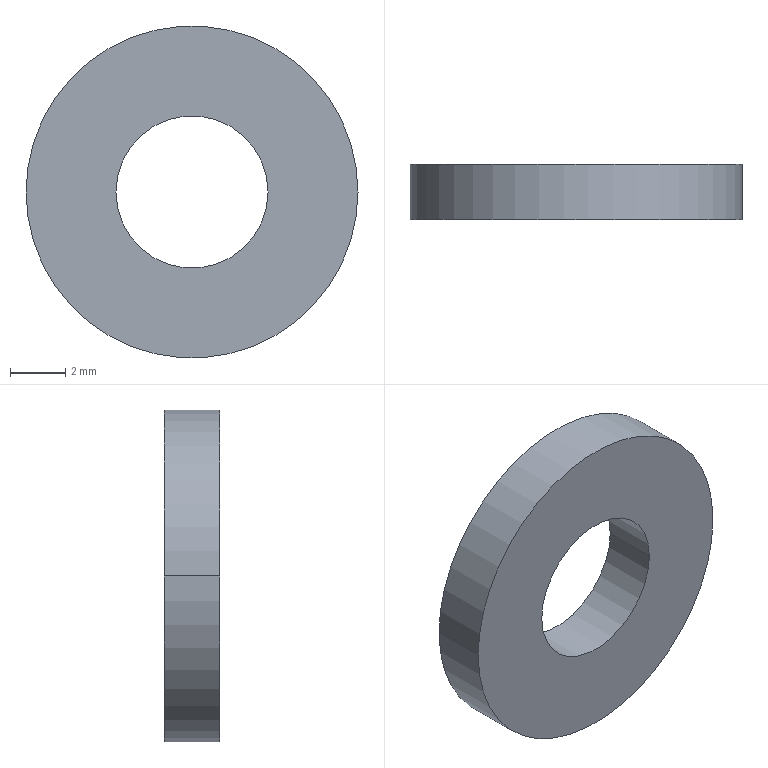Part | STEP file | WSX-SUS-M5X12-2-8 | 1 solid | 6 faces | box 12 x 2 x 12 mm | volume 178.678 mm3 | cylinder 4 | plane 2 | commonest cylinder face diameters 5.5 x2 12 x2
STEP:
#1=CARTESIAN_POINT('',(0.,0.,0.));
#2=DIRECTION('',(0.,0.,1.));
#3=DIRECTION('',(1.,0.,0.));
#4=AXIS2_PLACEMENT_3D('',#1,#2,#3);
#5=CARTESIAN_POINT('',(-2.75,0.,0.));
#6=VERTEX_POINT('',#5);
#7=CARTESIAN_POINT('',(-2.75,2.,0.));
#8=VERTEX_POINT('',#7);
#9=CARTESIAN_POINT('',(-2.75,0.,0.));
#10=DIRECTION('',(0.,1.,0.));
#11=VECTOR('',#10,1.);
#12=LINE('',#9,#11);
#13=CARTESIAN_POINT('',(0.,0.,0.));
#14=DIRECTION('',(0.,1.,0.));
#15=DIRECTION('',(-1.,0.,0.));
#16=AXIS2_PLACEMENT_3D('',#13,#14,#15);
#17=CYLINDRICAL_SURFACE('',#16,2.75);
#18=CARTESIAN_POINT('',(6.283,0.));
#19=DIRECTION('',(0.,1.));
#20=VECTOR('',#19,1.);
#21=LINE('',#18,#20);
#22=(GEOMETRIC_REPRESENTATION_CONTEXT(2)PARAMETRIC_REPRESENTATION_CONTEXT()REPRESENTATION_CONTEXT('',''));
#23=DEFINITIONAL_REPRESENTATION('',(#21),#22);
#24=PCURVE('',#17,#23);
#25=CARTESIAN_POINT('',(0.,0.,0.));
#26=DIRECTION('',(0.,1.,0.));
#27=DIRECTION('',(-1.,0.,0.));
#28=AXIS2_PLACEMENT_3D('',#25,#26,#27);
#29=CYLINDRICAL_SURFACE('',#28,2.75);
#30=CARTESIAN_POINT('',(0.,0.));
#31=DIRECTION('',(0.,1.));
#32=VECTOR('',#31,1.);
#33=LINE('',#30,#32);
#34=(GEOMETRIC_REPRESENTATION_CONTEXT(2)PARAMETRIC_REPRESENTATION_CONTEXT()REPRESENTATION_CONTEXT('',''));
#35=DEFINITIONAL_REPRESENTATION('',(#33),#34);
#36=PCURVE('',#29,#35);
#37=SURFACE_CURVE('',#12,(#24,#36),.PCURVE_S1.);
#38=EDGE_CURVE('',#6,#8,#37,.T.);
#39=ORIENTED_EDGE('',*,*,#38,.T.);
#40=CARTESIAN_POINT('',(2.75,2.,0.));
#41=VERTEX_POINT('',#40);
#42=CARTESIAN_POINT('',(0.,2.,0.));
#43=DIRECTION('',(0.,-1.,0.));
#44=DIRECTION('',(1.,0.,0.));
#45=AXIS2_PLACEMENT_3D('',#42,#43,#44);
#46=CIRCLE('',#45,2.75);
#47=CARTESIAN_POINT('',(9.425,2.));
#48=DIRECTION('',(-1.,0.));
#49=VECTOR('',#48,1.);
#50=LINE('',#47,#49);
#51=(GEOMETRIC_REPRESENTATION_CONTEXT(2)PARAMETRIC_REPRESENTATION_CONTEXT()REPRESENTATION_CONTEXT('',''));
#52=DEFINITIONAL_REPRESENTATION('',(#50),#51);
#53=PCURVE('',#17,#52);
#54=CARTESIAN_POINT('',(0.,2.,0.));
#55=DIRECTION('',(0.,1.,0.));
#56=DIRECTION('',(-1.,0.,0.));
#57=AXIS2_PLACEMENT_3D('',#54,#55,#56);
#58=PLANE('',#57);
#59=CARTESIAN_POINT('',(-2.75,0.));
#60=CARTESIAN_POINT('',(-2.75,4.763));
#61=CARTESIAN_POINT('',(1.375,2.382));
#62=CARTESIAN_POINT('',(5.5,0.));
#63=CARTESIAN_POINT('',(1.375,-2.382));
#64=CARTESIAN_POINT('',(-2.75,-4.763));
#65=CARTESIAN_POINT('',(-2.75,0.));
#66=(BOUNDED_CURVE()B_SPLINE_CURVE(2,(#59,#60,#61,#62,#63,#64,#65),.UNSPECIFIED.,.T.,.F.)B_SPLINE_CURVE_WITH_KNOTS((1,2,2,2,2,1),(-2.094,0.,2.094,4.189,6.283,8.378),.UNSPECIFIED.)CURVE()GEOMETRIC_REPRESENTATION_ITEM()RATIONAL_B_SPLINE_CURVE((1.,0.5,1.,0.5,1.,0.5,1.))REPRESENTATION_ITEM(''));
#67=(GEOMETRIC_REPRESENTATION_CONTEXT(2)PARAMETRIC_REPRESENTATION_CONTEXT()REPRESENTATION_CONTEXT('',''));
#68=DEFINITIONAL_REPRESENTATION('',(#66),#67);
#69=PCURVE('',#58,#68);
#70=SURFACE_CURVE('',#46,(#53,#69),.PCURVE_S1.);
#71=EDGE_CURVE('',#8,#41,#70,.T.);
#72=ORIENTED_EDGE('',*,*,#71,.T.);
#73=CARTESIAN_POINT('',(2.75,0.,0.));
#74=VERTEX_POINT('',#73);
#75=CARTESIAN_POINT('',(2.75,0.,0.));
#76=DIRECTION('',(0.,1.,0.));
#77=VECTOR('',#76,1.);
#78=LINE('',#75,#77);
#79=CARTESIAN_POINT('',(3.142,0.));
#80=DIRECTION('',(0.,1.));
#81=VECTOR('',#80,1.);
#82=LINE('',#79,#81);
#83=(GEOMETRIC_REPRESENTATION_CONTEXT(2)PARAMETRIC_REPRESENTATION_CONTEXT()REPRESENTATION_CONTEXT('',''));
#84=DEFINITIONAL_REPRESENTATION('',(#82),#83);
#85=PCURVE('',#17,#84);
#86=CARTESIAN_POINT('',(3.142,0.));
#87=DIRECTION('',(0.,1.));
#88=VECTOR('',#87,1.);
#89=LINE('',#86,#88);
#90=(GEOMETRIC_REPRESENTATION_CONTEXT(2)PARAMETRIC_REPRESENTATION_CONTEXT()REPRESENTATION_CONTEXT('',''));
#91=DEFINITIONAL_REPRESENTATION('',(#89),#90);
#92=PCURVE('',#29,#91);
#93=SURFACE_CURVE('',#78,(#85,#92),.PCURVE_S1.);
#94=EDGE_CURVE('',#74,#41,#93,.T.);
#95=ORIENTED_EDGE('',*,*,#94,.F.);
#96=CARTESIAN_POINT('',(0.,0.,0.));
#97=DIRECTION('',(0.,1.,0.));
#98=DIRECTION('',(-1.,0.,0.));
#99=AXIS2_PLACEMENT_3D('',#96,#97,#98);
#100=CIRCLE('',#99,2.75);
#101=CARTESIAN_POINT('',(0.,0.));
#102=DIRECTION('',(1.,0.));
#103=VECTOR('',#102,1.);
#104=LINE('',#101,#103);
#105=(GEOMETRIC_REPRESENTATION_CONTEXT(2)PARAMETRIC_REPRESENTATION_CONTEXT()REPRESENTATION_CONTEXT('',''));
#106=DEFINITIONAL_REPRESENTATION('',(#104),#105);
#107=PCURVE('',#17,#106);
#108=CARTESIAN_POINT('',(0.,0.,0.));
#109=DIRECTION('',(0.,-1.,0.));
#110=DIRECTION('',(1.,0.,0.));
#111=AXIS2_PLACEMENT_3D('',#108,#109,#110);
#112=PLANE('',#111);
#113=CARTESIAN_POINT('',(-2.75,0.));
#114=CARTESIAN_POINT('',(-2.75,4.763));
#115=CARTESIAN_POINT('',(1.375,2.382));
#116=CARTESIAN_POINT('',(5.5,0.));
#117=CARTESIAN_POINT('',(1.375,-2.382));
#118=CARTESIAN_POINT('',(-2.75,-4.763));
#119=CARTESIAN_POINT('',(-2.75,0.));
#120=(BOUNDED_CURVE()B_SPLINE_CURVE(2,(#113,#114,#115,#116,#117,#118,#119),.UNSPECIFIED.,.T.,.F.)B_SPLINE_CURVE_WITH_KNOTS((1,2,2,2,2,1),(-2.094,0.,2.094,4.189,6.283,8.378),.UNSPECIFIED.)CURVE()GEOMETRIC_REPRESENTATION_ITEM()RATIONAL_B_SPLINE_CURVE((1.,0.5,1.,0.5,1.,0.5,1.))REPRESENTATION_ITEM(''));
#121=(GEOMETRIC_REPRESENTATION_CONTEXT(2)PARAMETRIC_REPRESENTATION_CONTEXT()REPRESENTATION_CONTEXT('',''));
#122=DEFINITIONAL_REPRESENTATION('',(#120),#121);
#123=PCURVE('',#112,#122);
#124=SURFACE_CURVE('',#100,(#107,#123),.PCURVE_S1.);
#125=EDGE_CURVE('',#74,#6,#124,.T.);
#126=ORIENTED_EDGE('',*,*,#125,.T.);
#127=EDGE_LOOP('',(#39,#72,#95,#126));
#128=FACE_BOUND('',#127,.F.);
#129=ADVANCED_FACE('',(#128),#17,.F.);
#130=CARTESIAN_POINT('',(-6.,0.,0.));
#131=VERTEX_POINT('',#130);
#132=CARTESIAN_POINT('',(6.,0.,0.));
#133=VERTEX_POINT('',#132);
#134=CARTESIAN_POINT('',(0.,0.,0.));
#135=DIRECTION('',(0.,1.,0.));
#136=DIRECTION('',(-1.,0.,0.));
#137=AXIS2_PLACEMENT_3D('',#134,#135,#136);
#138=CIRCLE('',#137,6.);
#139=CARTESIAN_POINT('',(0.,0.,0.));
#140=DIRECTION('',(0.,1.,0.));
#141=DIRECTION('',(-1.,0.,0.));
#142=AXIS2_PLACEMENT_3D('',#139,#140,#141);
#143=CYLINDRICAL_SURFACE('',#142,6.);
#144=CARTESIAN_POINT('',(0.,0.));
#145=DIRECTION('',(1.,0.));
#146=VECTOR('',#145,1.);
#147=LINE('',#144,#146);
#148=(GEOMETRIC_REPRESENTATION_CONTEXT(2)PARAMETRIC_REPRESENTATION_CONTEXT()REPRESENTATION_CONTEXT('',''));
#149=DEFINITIONAL_REPRESENTATION('',(#147),#148);
#150=PCURVE('',#143,#149);
#151=CARTESIAN_POINT('',(-6.,0.));
#152=CARTESIAN_POINT('',(-6.,10.392));
#153=CARTESIAN_POINT('',(3.,5.196));
#154=CARTESIAN_POINT('',(12.,0.));
#155=CARTESIAN_POINT('',(3.,-5.196));
#156=CARTESIAN_POINT('',(-6.,-10.392));
#157=CARTESIAN_POINT('',(-6.,0.));
#158=(BOUNDED_CURVE()B_SPLINE_CURVE(2,(#151,#152,#153,#154,#155,#156,#157),.UNSPECIFIED.,.T.,.F.)B_SPLINE_CURVE_WITH_KNOTS((1,2,2,2,2,1),(-2.094,0.,2.094,4.189,6.283,8.378),.UNSPECIFIED.)CURVE()GEOMETRIC_REPRESENTATION_ITEM()RATIONAL_B_SPLINE_CURVE((1.,0.5,1.,0.5,1.,0.5,1.))REPRESENTATION_ITEM(''));
#159=(GEOMETRIC_REPRESENTATION_CONTEXT(2)PARAMETRIC_REPRESENTATION_CONTEXT()REPRESENTATION_CONTEXT('',''));
#160=DEFINITIONAL_REPRESENTATION('',(#158),#159);
#161=PCURVE('',#112,#160);
#162=SURFACE_CURVE('',#138,(#150,#161),.PCURVE_S1.);
#163=EDGE_CURVE('',#131,#133,#162,.T.);
#164=ORIENTED_EDGE('',*,*,#163,.T.);
#165=CARTESIAN_POINT('',(6.,2.,0.));
#166=VERTEX_POINT('',#165);
#167=CARTESIAN_POINT('',(6.,0.,0.));
#168=DIRECTION('',(0.,1.,0.));
#169=VECTOR('',#168,1.);
#170=LINE('',#167,#169);
#171=CARTESIAN_POINT('',(3.142,0.));
#172=DIRECTION('',(0.,1.));
#173=VECTOR('',#172,1.);
#174=LINE('',#171,#173);
#175=(GEOMETRIC_REPRESENTATION_CONTEXT(2)PARAMETRIC_REPRESENTATION_CONTEXT()REPRESENTATION_CONTEXT('',''));
#176=DEFINITIONAL_REPRESENTATION('',(#174),#175);
#177=PCURVE('',#143,#176);
#178=CARTESIAN_POINT('',(0.,0.,0.));
#179=DIRECTION('',(0.,1.,0.));
#180=DIRECTION('',(-1.,0.,0.));
#181=AXIS2_PLACEMENT_3D('',#178,#179,#180);
#182=CYLINDRICAL_SURFACE('',#181,6.);
#183=CARTESIAN_POINT('',(3.142,0.));
#184=DIRECTION('',(0.,1.));
#185=VECTOR('',#184,1.);
#186=LINE('',#183,#185);
#187=(GEOMETRIC_REPRESENTATION_CONTEXT(2)PARAMETRIC_REPRESENTATION_CONTEXT()REPRESENTATION_CONTEXT('',''));
#188=DEFINITIONAL_REPRESENTATION('',(#186),#187);
#189=PCURVE('',#182,#188);
#190=SURFACE_CURVE('',#170,(#177,#189),.PCURVE_S1.);
#191=EDGE_CURVE('',#133,#166,#190,.T.);
#192=ORIENTED_EDGE('',*,*,#191,.T.);
#193=CARTESIAN_POINT('',(-6.,2.,0.));
#194=VERTEX_POINT('',#193);
#195=CARTESIAN_POINT('',(0.,2.,0.));
#196=DIRECTION('',(0.,-1.,0.));
#197=DIRECTION('',(1.,0.,0.));
#198=AXIS2_PLACEMENT_3D('',#195,#196,#197);
#199=CIRCLE('',#198,6.);
#200=CARTESIAN_POINT('',(3.142,2.));
#201=DIRECTION('',(-1.,0.));
#202=VECTOR('',#201,1.);
#203=LINE('',#200,#202);
#204=(GEOMETRIC_REPRESENTATION_CONTEXT(2)PARAMETRIC_REPRESENTATION_CONTEXT()REPRESENTATION_CONTEXT('',''));
#205=DEFINITIONAL_REPRESENTATION('',(#203),#204);
#206=PCURVE('',#143,#205);
#207=CARTESIAN_POINT('',(-6.,0.));
#208=CARTESIAN_POINT('',(-6.,10.392));
#209=CARTESIAN_POINT('',(3.,5.196));
#210=CARTESIAN_POINT('',(12.,0.));
#211=CARTESIAN_POINT('',(3.,-5.196));
#212=CARTESIAN_POINT('',(-6.,-10.392));
#213=CARTESIAN_POINT('',(-6.,0.));
#214=(BOUNDED_CURVE()B_SPLINE_CURVE(2,(#207,#208,#209,#210,#211,#212,#213),.UNSPECIFIED.,.T.,.F.)B_SPLINE_CURVE_WITH_KNOTS((1,2,2,2,2,1),(-2.094,0.,2.094,4.189,6.283,8.378),.UNSPECIFIED.)CURVE()GEOMETRIC_REPRESENTATION_ITEM()RATIONAL_B_SPLINE_CURVE((1.,0.5,1.,0.5,1.,0.5,1.))REPRESENTATION_ITEM(''));
#215=(GEOMETRIC_REPRESENTATION_CONTEXT(2)PARAMETRIC_REPRESENTATION_CONTEXT()REPRESENTATION_CONTEXT('',''));
#216=DEFINITIONAL_REPRESENTATION('',(#214),#215);
#217=PCURVE('',#58,#216);
#218=SURFACE_CURVE('',#199,(#206,#217),.PCURVE_S1.);
#219=EDGE_CURVE('',#166,#194,#218,.T.);
#220=ORIENTED_EDGE('',*,*,#219,.T.);
#221=CARTESIAN_POINT('',(-6.,0.,0.));
#222=DIRECTION('',(0.,1.,0.));
#223=VECTOR('',#222,1.);
#224=LINE('',#221,#223);
#225=CARTESIAN_POINT('',(0.,0.));
#226=DIRECTION('',(0.,1.));
#227=VECTOR('',#226,1.);
#228=LINE('',#225,#227);
#229=(GEOMETRIC_REPRESENTATION_CONTEXT(2)PARAMETRIC_REPRESENTATION_CONTEXT()REPRESENTATION_CONTEXT('',''));
#230=DEFINITIONAL_REPRESENTATION('',(#228),#229);
#231=PCURVE('',#143,#230);
#232=CARTESIAN_POINT('',(6.283,0.));
#233=DIRECTION('',(0.,1.));
#234=VECTOR('',#233,1.);
#235=LINE('',#232,#234);
#236=(GEOMETRIC_REPRESENTATION_CONTEXT(2)PARAMETRIC_REPRESENTATION_CONTEXT()REPRESENTATION_CONTEXT('',''));
#237=DEFINITIONAL_REPRESENTATION('',(#235),#236);
#238=PCURVE('',#182,#237);
#239=SURFACE_CURVE('',#224,(#231,#238),.PCURVE_S1.);
#240=EDGE_CURVE('',#131,#194,#239,.T.);
#241=ORIENTED_EDGE('',*,*,#240,.F.);
#242=EDGE_LOOP('',(#164,#192,#220,#241));
#243=FACE_BOUND('',#242,.T.);
#244=ADVANCED_FACE('',(#243),#143,.T.);
#245=ORIENTED_EDGE('',*,*,#71,.T.);
#246=CARTESIAN_POINT('',(0.,2.,0.));
#247=DIRECTION('',(0.,-1.,0.));
#248=DIRECTION('',(1.,0.,0.));
#249=AXIS2_PLACEMENT_3D('',#246,#247,#248);
#250=CIRCLE('',#249,2.75);
#251=CARTESIAN_POINT('',(-2.75,0.));
#252=CARTESIAN_POINT('',(-2.75,4.763));
#253=CARTESIAN_POINT('',(1.375,2.382));
#254=CARTESIAN_POINT('',(5.5,0.));
#255=CARTESIAN_POINT('',(1.375,-2.382));
#256=CARTESIAN_POINT('',(-2.75,-4.763));
#257=CARTESIAN_POINT('',(-2.75,0.));
#258=(BOUNDED_CURVE()B_SPLINE_CURVE(2,(#251,#252,#253,#254,#255,#256,#257),.UNSPECIFIED.,.T.,.F.)B_SPLINE_CURVE_WITH_KNOTS((1,2,2,2,2,1),(-2.094,0.,2.094,4.189,6.283,8.378),.UNSPECIFIED.)CURVE()GEOMETRIC_REPRESENTATION_ITEM()RATIONAL_B_SPLINE_CURVE((1.,0.5,1.,0.5,1.,0.5,1.))REPRESENTATION_ITEM(''));
#259=(GEOMETRIC_REPRESENTATION_CONTEXT(2)PARAMETRIC_REPRESENTATION_CONTEXT()REPRESENTATION_CONTEXT('',''));
#260=DEFINITIONAL_REPRESENTATION('',(#258),#259);
#261=PCURVE('',#58,#260);
#262=CARTESIAN_POINT('',(3.142,2.));
#263=DIRECTION('',(-1.,0.));
#264=VECTOR('',#263,1.);
#265=LINE('',#262,#264);
#266=(GEOMETRIC_REPRESENTATION_CONTEXT(2)PARAMETRIC_REPRESENTATION_CONTEXT()REPRESENTATION_CONTEXT('',''));
#267=DEFINITIONAL_REPRESENTATION('',(#265),#266);
#268=PCURVE('',#29,#267);
#269=SURFACE_CURVE('',#250,(#261,#268),.PCURVE_S1.);
#270=EDGE_CURVE('',#41,#8,#269,.T.);
#271=ORIENTED_EDGE('',*,*,#270,.T.);
#272=EDGE_LOOP('',(#245,#271));
#273=FACE_BOUND('',#272,.T.);
#274=CARTESIAN_POINT('',(0.,2.,0.));
#275=DIRECTION('',(0.,-1.,0.));
#276=DIRECTION('',(1.,0.,0.));
#277=AXIS2_PLACEMENT_3D('',#274,#275,#276);
#278=CIRCLE('',#277,6.);
#279=CARTESIAN_POINT('',(-6.,0.));
#280=CARTESIAN_POINT('',(-6.,10.392));
#281=CARTESIAN_POINT('',(3.,5.196));
#282=CARTESIAN_POINT('',(12.,0.));
#283=CARTESIAN_POINT('',(3.,-5.196));
#284=CARTESIAN_POINT('',(-6.,-10.392));
#285=CARTESIAN_POINT('',(-6.,0.));
#286=(BOUNDED_CURVE()B_SPLINE_CURVE(2,(#279,#280,#281,#282,#283,#284,#285),.UNSPECIFIED.,.T.,.F.)B_SPLINE_CURVE_WITH_KNOTS((1,2,2,2,2,1),(-2.094,0.,2.094,4.189,6.283,8.378),.UNSPECIFIED.)CURVE()GEOMETRIC_REPRESENTATION_ITEM()RATIONAL_B_SPLINE_CURVE((1.,0.5,1.,0.5,1.,0.5,1.))REPRESENTATION_ITEM(''));
#287=(GEOMETRIC_REPRESENTATION_CONTEXT(2)PARAMETRIC_REPRESENTATION_CONTEXT()REPRESENTATION_CONTEXT('',''));
#288=DEFINITIONAL_REPRESENTATION('',(#286),#287);
#289=PCURVE('',#58,#288);
#290=CARTESIAN_POINT('',(9.425,2.));
#291=DIRECTION('',(-1.,0.));
#292=VECTOR('',#291,1.);
#293=LINE('',#290,#292);
#294=(GEOMETRIC_REPRESENTATION_CONTEXT(2)PARAMETRIC_REPRESENTATION_CONTEXT()REPRESENTATION_CONTEXT('',''));
#295=DEFINITIONAL_REPRESENTATION('',(#293),#294);
#296=PCURVE('',#182,#295);
#297=SURFACE_CURVE('',#278,(#289,#296),.PCURVE_S1.);
#298=EDGE_CURVE('',#194,#166,#297,.T.);
#299=ORIENTED_EDGE('',*,*,#298,.F.);
#300=ORIENTED_EDGE('',*,*,#219,.F.);
#301=EDGE_LOOP('',(#299,#300));
#302=FACE_BOUND('',#301,.T.);
#303=ADVANCED_FACE('',(#273,#302),#58,.T.);
#304=CARTESIAN_POINT('',(0.,0.,0.));
#305=DIRECTION('',(0.,1.,0.));
#306=DIRECTION('',(-1.,0.,0.));
#307=AXIS2_PLACEMENT_3D('',#304,#305,#306);
#308=CIRCLE('',#307,2.75);
#309=CARTESIAN_POINT('',(-2.75,0.));
#310=CARTESIAN_POINT('',(-2.75,4.763));
#311=CARTESIAN_POINT('',(1.375,2.382));
#312=CARTESIAN_POINT('',(5.5,0.));
#313=CARTESIAN_POINT('',(1.375,-2.382));
#314=CARTESIAN_POINT('',(-2.75,-4.763));
#315=CARTESIAN_POINT('',(-2.75,0.));
#316=(BOUNDED_CURVE()B_SPLINE_CURVE(2,(#309,#310,#311,#312,#313,#314,#315),.UNSPECIFIED.,.T.,.F.)B_SPLINE_CURVE_WITH_KNOTS((1,2,2,2,2,1),(-2.094,0.,2.094,4.189,6.283,8.378),.UNSPECIFIED.)CURVE()GEOMETRIC_REPRESENTATION_ITEM()RATIONAL_B_SPLINE_CURVE((1.,0.5,1.,0.5,1.,0.5,1.))REPRESENTATION_ITEM(''));
#317=(GEOMETRIC_REPRESENTATION_CONTEXT(2)PARAMETRIC_REPRESENTATION_CONTEXT()REPRESENTATION_CONTEXT('',''));
#318=DEFINITIONAL_REPRESENTATION('',(#316),#317);
#319=PCURVE('',#112,#318);
#320=CARTESIAN_POINT('',(0.,0.));
#321=DIRECTION('',(1.,0.));
#322=VECTOR('',#321,1.);
#323=LINE('',#320,#322);
#324=(GEOMETRIC_REPRESENTATION_CONTEXT(2)PARAMETRIC_REPRESENTATION_CONTEXT()REPRESENTATION_CONTEXT('',''));
#325=DEFINITIONAL_REPRESENTATION('',(#323),#324);
#326=PCURVE('',#29,#325);
#327=SURFACE_CURVE('',#308,(#319,#326),.PCURVE_S1.);
#328=EDGE_CURVE('',#6,#74,#327,.T.);
#329=ORIENTED_EDGE('',*,*,#328,.T.);
#330=ORIENTED_EDGE('',*,*,#125,.T.);
#331=EDGE_LOOP('',(#329,#330));
#332=FACE_BOUND('',#331,.T.);
#333=ORIENTED_EDGE('',*,*,#163,.F.);
#334=CARTESIAN_POINT('',(0.,0.,0.));
#335=DIRECTION('',(0.,1.,0.));
#336=DIRECTION('',(-1.,0.,0.));
#337=AXIS2_PLACEMENT_3D('',#334,#335,#336);
#338=CIRCLE('',#337,6.);
#339=CARTESIAN_POINT('',(-6.,0.));
#340=CARTESIAN_POINT('',(-6.,10.392));
#341=CARTESIAN_POINT('',(3.,5.196));
#342=CARTESIAN_POINT('',(12.,0.));
#343=CARTESIAN_POINT('',(3.,-5.196));
#344=CARTESIAN_POINT('',(-6.,-10.392));
#345=CARTESIAN_POINT('',(-6.,0.));
#346=(BOUNDED_CURVE()B_SPLINE_CURVE(2,(#339,#340,#341,#342,#343,#344,#345),.UNSPECIFIED.,.T.,.F.)B_SPLINE_CURVE_WITH_KNOTS((1,2,2,2,2,1),(-2.094,0.,2.094,4.189,6.283,8.378),.UNSPECIFIED.)CURVE()GEOMETRIC_REPRESENTATION_ITEM()RATIONAL_B_SPLINE_CURVE((1.,0.5,1.,0.5,1.,0.5,1.))REPRESENTATION_ITEM(''));
#347=(GEOMETRIC_REPRESENTATION_CONTEXT(2)PARAMETRIC_REPRESENTATION_CONTEXT()REPRESENTATION_CONTEXT('',''));
#348=DEFINITIONAL_REPRESENTATION('',(#346),#347);
#349=PCURVE('',#112,#348);
#350=CARTESIAN_POINT('',(0.,0.));
#351=DIRECTION('',(1.,0.));
#352=VECTOR('',#351,1.);
#353=LINE('',#350,#352);
#354=(GEOMETRIC_REPRESENTATION_CONTEXT(2)PARAMETRIC_REPRESENTATION_CONTEXT()REPRESENTATION_CONTEXT('',''));
#355=DEFINITIONAL_REPRESENTATION('',(#353),#354);
#356=PCURVE('',#182,#355);
#357=SURFACE_CURVE('',#338,(#349,#356),.PCURVE_S1.);
#358=EDGE_CURVE('',#133,#131,#357,.T.);
#359=ORIENTED_EDGE('',*,*,#358,.F.);
#360=EDGE_LOOP('',(#333,#359));
#361=FACE_BOUND('',#360,.T.);
#362=ADVANCED_FACE('',(#332,#361),#112,.T.);
#363=ORIENTED_EDGE('',*,*,#191,.F.);
#364=ORIENTED_EDGE('',*,*,#358,.T.);
#365=ORIENTED_EDGE('',*,*,#240,.T.);
#366=ORIENTED_EDGE('',*,*,#298,.T.);
#367=EDGE_LOOP('',(#363,#364,#365,#366));
#368=FACE_BOUND('',#367,.T.);
#369=ADVANCED_FACE('',(#368),#182,.T.);
#370=ORIENTED_EDGE('',*,*,#270,.T.);
#371=ORIENTED_EDGE('',*,*,#38,.F.);
#372=ORIENTED_EDGE('',*,*,#328,.T.);
#373=ORIENTED_EDGE('',*,*,#94,.T.);
#374=EDGE_LOOP('',(#370,#371,#372,#373));
#375=FACE_BOUND('',#374,.F.);
#376=ADVANCED_FACE('',(#375),#29,.F.);
#377=CLOSED_SHELL('',(#129,#244,#303,#362,#369,#376));
#378=MANIFOLD_SOLID_BREP('',#377);
#379=(LENGTH_UNIT()NAMED_UNIT(*)SI_UNIT(.MILLI.,.METRE.));
#380=UNCERTAINTY_MEASURE_WITH_UNIT(LENGTH_MEASURE(0.0000001),#379,'','');
#381=(NAMED_UNIT(*)PLANE_ANGLE_UNIT()SI_UNIT($,.RADIAN.));
#382=(NAMED_UNIT(*)SI_UNIT($,.STERADIAN.)SOLID_ANGLE_UNIT());
#383=(GEOMETRIC_REPRESENTATION_CONTEXT(3)GLOBAL_UNCERTAINTY_ASSIGNED_CONTEXT((#380))GLOBAL_UNIT_ASSIGNED_CONTEXT((#379,#381,#382))REPRESENTATION_CONTEXT('',''));
#384=ADVANCED_BREP_SHAPE_REPRESENTATION('',(#4,#378),#383);